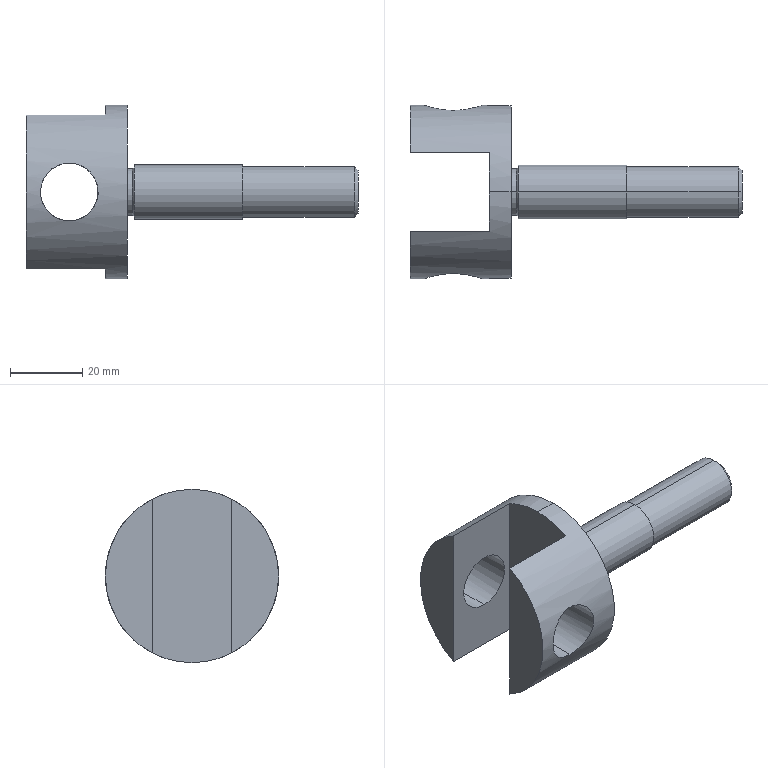Part | SolidWorks | features ICE 2, Chamfer 1, RevCut 1, Revolution 1 | 1 solid | 30 faces | box 92 x 48 x 48 mm | volume 33624 mm3 | cylinder 12 | plane 10 | cone 6 | torus 2 | commonest cylinder face diameters 16 x4 13 x2 14 x2 15 x2 48 x2
STEP:
#1=CARTESIAN_POINT('',(92.,0.,-6.));
#2=VERTEX_POINT('',#1);
#3=CARTESIAN_POINT('',(92.,0.,6.));
#4=VERTEX_POINT('',#3);
#5=CARTESIAN_POINT('',(92.,0.,0.));
#6=DIRECTION('',(1.,0.,0.));
#7=DIRECTION('',(0.,0.,1.));
#8=AXIS2_PLACEMENT_3D('',#5,#6,#7);
#9=CIRCLE('',#8,6.);
#10=EDGE_CURVE('',#2,#4,#9,.T.);
#11=ORIENTED_EDGE('',*,*,#10,.F.);
#12=CARTESIAN_POINT('',(91.,0.,-7.));
#13=VERTEX_POINT('',#12);
#14=CARTESIAN_POINT('',(91.,0.,-7.));
#15=DIRECTION('',(-0.7071,0.,-0.7071));
#16=VECTOR('',#15,1000.);
#17=LINE('',#14,#16);
#18=EDGE_CURVE('',#2,#13,#17,.T.);
#19=ORIENTED_EDGE('',*,*,#18,.T.);
#20=CARTESIAN_POINT('',(91.,0.,7.));
#21=VERTEX_POINT('',#20);
#22=CARTESIAN_POINT('',(91.,0.,0.));
#23=DIRECTION('',(-1.,0.,0.));
#24=DIRECTION('',(0.,0.,1.));
#25=AXIS2_PLACEMENT_3D('',#22,#23,#24);
#26=CIRCLE('',#25,7.);
#27=EDGE_CURVE('',#21,#13,#26,.T.);
#28=ORIENTED_EDGE('',*,*,#27,.F.);
#29=CARTESIAN_POINT('',(91.,0.,7.));
#30=DIRECTION('',(-0.7071,0.,0.7071));
#31=VECTOR('',#30,1000.);
#32=LINE('',#29,#31);
#33=EDGE_CURVE('',#4,#21,#32,.T.);
#34=ORIENTED_EDGE('',*,*,#33,.F.);
#35=EDGE_LOOP('',(#11,#19,#28,#34));
#36=FACE_OUTER_BOUND('',#35,.T.);
#37=CARTESIAN_POINT('',(91.,0.,0.));
#38=DIRECTION('',(-1.,0.,0.));
#39=DIRECTION('',(0.,0.,1.));
#40=AXIS2_PLACEMENT_3D('',#37,#38,#39);
#41=CONICAL_SURFACE('',#40,7.,0.7854);
#42=ADVANCED_FACE('',(#36),#41,.T.);
#43=CARTESIAN_POINT('',(12.,22.627,-8.));
#44=VERTEX_POINT('',#43);
#45=CARTESIAN_POINT('',(12.,22.627,8.));
#46=VERTEX_POINT('',#45);
#47=CARTESIAN_POINT('',(12.,22.627,-8.));
#48=CARTESIAN_POINT('',(11.467,22.627,-8.));
#49=CARTESIAN_POINT('',(10.944,22.646,-7.947));
#50=CARTESIAN_POINT('',(10.174,22.7,-7.793));
#51=CARTESIAN_POINT('',(9.919,22.722,-7.729));
#52=CARTESIAN_POINT('',(9.414,22.773,-7.575));
#53=CARTESIAN_POINT('',(9.165,22.803,-7.485));
#54=CARTESIAN_POINT('',(8.44,22.901,-7.183));
#55=CARTESIAN_POINT('',(7.982,22.977,-6.937));
#56=CARTESIAN_POINT('',(7.332,23.103,-6.502));
#57=CARTESIAN_POINT('',(7.12,23.147,-6.345));
#58=CARTESIAN_POINT('',(6.717,23.235,-6.013));
#59=CARTESIAN_POINT('',(6.525,23.28,-5.839));
#60=CARTESIAN_POINT('',(5.976,23.413,-5.29));
#61=CARTESIAN_POINT('',(5.646,23.501,-4.889));
#62=CARTESIAN_POINT('',(5.061,23.666,-4.016));
#63=CARTESIAN_POINT('',(4.815,23.74,-3.556));
#64=CARTESIAN_POINT('',(4.515,23.833,-2.835));
#65=CARTESIAN_POINT('',(4.426,23.861,-2.589));
#66=CARTESIAN_POINT('',(4.272,23.91,-2.086));
#67=CARTESIAN_POINT('',(4.207,23.932,-1.828));
#68=CARTESIAN_POINT('',(4.052,23.983,-1.052));
#69=CARTESIAN_POINT('',(4.,24.,-0.5299));
#70=CARTESIAN_POINT('',(4.,24.,0.5225));
#71=CARTESIAN_POINT('',(4.053,23.982,1.057));
#72=CARTESIAN_POINT('',(4.259,23.915,2.086));
#73=CARTESIAN_POINT('',(4.412,23.865,2.587));
#74=CARTESIAN_POINT('',(4.817,23.739,3.561));
#75=CARTESIAN_POINT('',(5.065,23.665,4.023));
#76=CARTESIAN_POINT('',(5.499,23.542,4.67));
#77=CARTESIAN_POINT('',(5.654,23.5,4.878));
#78=CARTESIAN_POINT('',(5.986,23.413,5.282));
#79=CARTESIAN_POINT('',(6.163,23.368,5.477));
#80=CARTESIAN_POINT('',(6.715,23.234,6.029));
#81=CARTESIAN_POINT('',(7.115,23.145,6.357));
#82=CARTESIAN_POINT('',(7.979,22.978,6.936));
#83=CARTESIAN_POINT('',(8.447,22.9,7.187));
#84=CARTESIAN_POINT('',(9.41,22.77,7.587));
#85=CARTESIAN_POINT('',(9.909,22.718,7.74));
#86=CARTESIAN_POINT('',(10.686,22.664,7.896));
#87=CARTESIAN_POINT('',(10.95,22.65,7.935));
#88=CARTESIAN_POINT('',(11.475,22.632,7.987));
#89=CARTESIAN_POINT('',(11.738,22.627,8.));
#90=CARTESIAN_POINT('',(12.,22.627,8.));
#91=B_SPLINE_CURVE_WITH_KNOTS('',3,(#47,#48,#49,#50,#51,#52,#53,#54,#55,#56,#57,#58,#59,#60,#61,#62,#63,#64,#65,#66,#67,#68,#69,#70,#71,#72,#73,#74,#75,#76,#77,#78,#79,#80,#81,#82,#83,#84,#85,#86,#87,#88,#89,#90),.UNSPECIFIED.,.F.,.F.,(4,2,2,2,2,2,2,2,2,2,2,2,2,2,2,2,2,2,2,2,2,4),(0.,0.001575,0.002362,0.003149,0.004724,0.005511,0.006298,0.007873,0.009447,0.01023,0.01102,0.0126,0.01417,0.01575,0.01732,0.01811,0.01889,0.02047,0.02204,0.02362,0.02441,0.02519),.UNSPECIFIED.);
#92=EDGE_CURVE('',#44,#46,#91,.T.);
#93=ORIENTED_EDGE('',*,*,#92,.F.);
#94=CARTESIAN_POINT('',(12.,22.627,8.));
#95=CARTESIAN_POINT('',(12.262,22.627,8.));
#96=CARTESIAN_POINT('',(12.524,22.632,7.987));
#97=CARTESIAN_POINT('',(13.049,22.65,7.935));
#98=CARTESIAN_POINT('',(13.312,22.664,7.896));
#99=CARTESIAN_POINT('',(14.09,22.718,7.74));
#100=CARTESIAN_POINT('',(14.591,22.77,7.587));
#101=CARTESIAN_POINT('',(15.556,22.9,7.186));
#102=CARTESIAN_POINT('',(16.023,22.978,6.934));
#103=CARTESIAN_POINT('',(16.886,23.145,6.356));
#104=CARTESIAN_POINT('',(17.287,23.234,6.027));
#105=CARTESIAN_POINT('',(17.841,23.369,5.473));
#106=CARTESIAN_POINT('',(18.018,23.413,5.278));
#107=CARTESIAN_POINT('',(18.348,23.5,4.876));
#108=CARTESIAN_POINT('',(18.502,23.543,4.668));
#109=CARTESIAN_POINT('',(18.791,23.624,4.237));
#110=CARTESIAN_POINT('',(18.925,23.663,4.015));
#111=CARTESIAN_POINT('',(19.172,23.736,3.555));
#112=CARTESIAN_POINT('',(19.285,23.771,3.316));
#113=CARTESIAN_POINT('',(19.589,23.865,2.587));
#114=CARTESIAN_POINT('',(19.741,23.915,2.087));
#115=CARTESIAN_POINT('',(19.895,23.965,1.316));
#116=CARTESIAN_POINT('',(19.934,23.978,1.056));
#117=CARTESIAN_POINT('',(19.987,23.996,0.5287));
#118=CARTESIAN_POINT('',(20.,24.,0.2624));
#119=CARTESIAN_POINT('',(20.,24.,-0.5283));
#120=CARTESIAN_POINT('',(19.948,23.983,-1.05));
#121=CARTESIAN_POINT('',(19.793,23.932,-1.826));
#122=CARTESIAN_POINT('',(19.728,23.911,-2.084));
#123=CARTESIAN_POINT('',(19.574,23.861,-2.588));
#124=CARTESIAN_POINT('',(19.486,23.833,-2.835));
#125=CARTESIAN_POINT('',(19.285,23.771,-3.316));
#126=CARTESIAN_POINT('',(19.173,23.737,-3.552));
#127=CARTESIAN_POINT('',(18.926,23.663,-4.012));
#128=CARTESIAN_POINT('',(18.791,23.624,-4.238));
#129=CARTESIAN_POINT('',(18.353,23.501,-4.891));
#130=CARTESIAN_POINT('',(18.023,23.413,-5.291));
#131=CARTESIAN_POINT('',(17.29,23.235,-6.024));
#132=CARTESIAN_POINT('',(16.881,23.144,-6.36));
#133=CARTESIAN_POINT('',(16.017,22.977,-6.938));
#134=CARTESIAN_POINT('',(15.56,22.901,-7.184));
#135=CARTESIAN_POINT('',(14.835,22.803,-7.486));
#136=CARTESIAN_POINT('',(14.585,22.773,-7.575));
#137=CARTESIAN_POINT('',(14.081,22.721,-7.729));
#138=CARTESIAN_POINT('',(13.826,22.7,-7.793));
#139=CARTESIAN_POINT('',(13.056,22.646,-7.947));
#140=CARTESIAN_POINT('',(12.533,22.627,-8.));
#141=CARTESIAN_POINT('',(12.,22.627,-8.));
#142=B_SPLINE_CURVE_WITH_KNOTS('',3,(#94,#95,#96,#97,#98,#99,#100,#101,#102,#103,#104,#105,#106,#107,#108,#109,#110,#111,#112,#113,#114,#115,#116,#117,#118,#119,#120,#121,#122,#123,#124,#125,#126,#127,#128,#129,#130,#131,#132,#133,#134,#135,#136,#137,#138,#139,#140,#141),.UNSPECIFIED.,.F.,.F.,(4,2,2,2,2,2,2,2,2,2,2,2,2,2,2,2,2,2,2,2,2,2,2,4),(0.02519,0.02598,0.02677,0.02834,0.02991,0.03149,0.03228,0.03306,0.03385,0.03464,0.03621,0.037,0.03779,0.03936,0.04015,0.04093,0.04172,0.04251,0.04408,0.04566,0.04723,0.04802,0.0488,0.05038),.UNSPECIFIED.);
#143=EDGE_CURVE('',#46,#44,#142,.T.);
#144=ORIENTED_EDGE('',*,*,#143,.F.);
#145=EDGE_LOOP('',(#93,#144));
#146=FACE_BOUND('',#145,.T.);
#147=CARTESIAN_POINT('',(28.,0.,24.));
#148=VERTEX_POINT('',#147);
#149=CARTESIAN_POINT('',(28.,0.,-24.));
#150=VERTEX_POINT('',#149);
#151=CARTESIAN_POINT('',(28.,0.,0.));
#152=DIRECTION('',(-1.,0.,0.));
#153=DIRECTION('',(0.,0.,1.));
#154=AXIS2_PLACEMENT_3D('',#151,#152,#153);
#155=CIRCLE('',#154,24.);
#156=EDGE_CURVE('',#148,#150,#155,.T.);
#157=ORIENTED_EDGE('',*,*,#156,.T.);
#158=CARTESIAN_POINT('',(22.,0.,-24.));
#159=VERTEX_POINT('',#158);
#160=CARTESIAN_POINT('',(-36.182,0.,-24.));
#161=DIRECTION('',(-1.,0.,0.));
#162=VECTOR('',#161,1000.);
#163=LINE('',#160,#162);
#164=EDGE_CURVE('',#150,#159,#163,.T.);
#165=ORIENTED_EDGE('',*,*,#164,.T.);
#166=CARTESIAN_POINT('',(22.,11.,-21.331));
#167=VERTEX_POINT('',#166);
#168=CARTESIAN_POINT('',(22.,0.,0.));
#169=DIRECTION('',(-1.,0.,0.));
#170=DIRECTION('',(0.,0.,1.));
#171=AXIS2_PLACEMENT_3D('',#168,#169,#170);
#172=CIRCLE('',#171,24.);
#173=EDGE_CURVE('',#167,#159,#172,.T.);
#174=ORIENTED_EDGE('',*,*,#173,.F.);
#175=CARTESIAN_POINT('',(0.,11.,-21.331));
#176=VERTEX_POINT('',#175);
#177=CARTESIAN_POINT('',(-36.182,11.,-21.331));
#178=DIRECTION('',(-1.,0.,0.));
#179=VECTOR('',#178,1000.);
#180=LINE('',#177,#179);
#181=EDGE_CURVE('',#167,#176,#180,.T.);
#182=ORIENTED_EDGE('',*,*,#181,.T.);
#183=CARTESIAN_POINT('',(0.,11.,21.331));
#184=VERTEX_POINT('',#183);
#185=CARTESIAN_POINT('',(0.,0.,0.));
#186=DIRECTION('',(-1.,0.,0.));
#187=DIRECTION('',(0.,0.,1.));
#188=AXIS2_PLACEMENT_3D('',#185,#186,#187);
#189=CIRCLE('',#188,24.);
#190=EDGE_CURVE('',#184,#176,#189,.T.);
#191=ORIENTED_EDGE('',*,*,#190,.F.);
#192=CARTESIAN_POINT('',(22.,11.,21.331));
#193=VERTEX_POINT('',#192);
#194=CARTESIAN_POINT('',(-36.182,11.,21.331));
#195=DIRECTION('',(1.,0.,0.));
#196=VECTOR('',#195,1000.);
#197=LINE('',#194,#196);
#198=EDGE_CURVE('',#184,#193,#197,.T.);
#199=ORIENTED_EDGE('',*,*,#198,.T.);
#200=CARTESIAN_POINT('',(22.,0.,24.));
#201=VERTEX_POINT('',#200);
#202=CARTESIAN_POINT('',(22.,0.,0.));
#203=DIRECTION('',(-1.,0.,0.));
#204=DIRECTION('',(0.,0.,1.));
#205=AXIS2_PLACEMENT_3D('',#202,#203,#204);
#206=CIRCLE('',#205,24.);
#207=EDGE_CURVE('',#201,#193,#206,.T.);
#208=ORIENTED_EDGE('',*,*,#207,.F.);
#209=CARTESIAN_POINT('',(-36.182,0.,24.));
#210=DIRECTION('',(-1.,0.,0.));
#211=VECTOR('',#210,1000.);
#212=LINE('',#209,#211);
#213=EDGE_CURVE('',#148,#201,#212,.T.);
#214=ORIENTED_EDGE('',*,*,#213,.F.);
#215=EDGE_LOOP('',(#157,#165,#174,#182,#191,#199,#208,#214));
#216=FACE_OUTER_BOUND('',#215,.T.);
#217=CARTESIAN_POINT('',(-36.182,0.,0.));
#218=DIRECTION('',(-1.,0.,0.));
#219=DIRECTION('',(0.,0.,1.));
#220=AXIS2_PLACEMENT_3D('',#217,#218,#219);
#221=CYLINDRICAL_SURFACE('',#220,24.);
#222=ADVANCED_FACE('',(#146,#216),#221,.T.);
#223=CARTESIAN_POINT('',(12.,-11.,-8.));
#224=VERTEX_POINT('',#223);
#225=CARTESIAN_POINT('',(12.,-11.,8.));
#226=VERTEX_POINT('',#225);
#227=CARTESIAN_POINT('',(12.,-11.,0.));
#228=DIRECTION('',(0.,1.,0.));
#229=DIRECTION('',(0.,0.,-1.));
#230=AXIS2_PLACEMENT_3D('',#227,#228,#229);
#231=CIRCLE('',#230,8.);
#232=EDGE_CURVE('',#224,#226,#231,.T.);
#233=ORIENTED_EDGE('',*,*,#232,.T.);
#234=CARTESIAN_POINT('',(12.,-22.627,8.));
#235=VERTEX_POINT('',#234);
#236=CARTESIAN_POINT('',(12.,40.,8.));
#237=DIRECTION('',(0.,-1.,0.));
#238=VECTOR('',#237,1000.);
#239=LINE('',#236,#238);
#240=EDGE_CURVE('',#226,#235,#239,.T.);
#241=ORIENTED_EDGE('',*,*,#240,.T.);
#242=CARTESIAN_POINT('',(12.,-22.627,-8.));
#243=VERTEX_POINT('',#242);
#244=CARTESIAN_POINT('',(12.,-22.627,8.));
#245=CARTESIAN_POINT('',(11.738,-22.627,8.));
#246=CARTESIAN_POINT('',(11.476,-22.632,7.987));
#247=CARTESIAN_POINT('',(10.951,-22.65,7.935));
#248=CARTESIAN_POINT('',(10.688,-22.664,7.896));
#249=CARTESIAN_POINT('',(9.91,-22.718,7.74));
#250=CARTESIAN_POINT('',(9.409,-22.77,7.587));
#251=CARTESIAN_POINT('',(8.444,-22.9,7.186));
#252=CARTESIAN_POINT('',(7.977,-22.978,6.934));
#253=CARTESIAN_POINT('',(7.114,-23.145,6.356));
#254=CARTESIAN_POINT('',(6.713,-23.234,6.027));
#255=CARTESIAN_POINT('',(6.159,-23.369,5.473));
#256=CARTESIAN_POINT('',(5.982,-23.413,5.278));
#257=CARTESIAN_POINT('',(5.652,-23.5,4.876));
#258=CARTESIAN_POINT('',(5.498,-23.543,4.668));
#259=CARTESIAN_POINT('',(5.209,-23.624,4.237));
#260=CARTESIAN_POINT('',(5.075,-23.663,4.015));
#261=CARTESIAN_POINT('',(4.828,-23.736,3.555));
#262=CARTESIAN_POINT('',(4.715,-23.771,3.316));
#263=CARTESIAN_POINT('',(4.411,-23.865,2.587));
#264=CARTESIAN_POINT('',(4.259,-23.915,2.087));
#265=CARTESIAN_POINT('',(4.105,-23.965,1.316));
#266=CARTESIAN_POINT('',(4.066,-23.978,1.056));
#267=CARTESIAN_POINT('',(4.013,-23.996,0.5287));
#268=CARTESIAN_POINT('',(4.,-24.,0.2624));
#269=CARTESIAN_POINT('',(4.,-24.,-0.5283));
#270=CARTESIAN_POINT('',(4.052,-23.983,-1.05));
#271=CARTESIAN_POINT('',(4.207,-23.932,-1.826));
#272=CARTESIAN_POINT('',(4.272,-23.911,-2.084));
#273=CARTESIAN_POINT('',(4.426,-23.861,-2.588));
#274=CARTESIAN_POINT('',(4.514,-23.833,-2.835));
#275=CARTESIAN_POINT('',(4.715,-23.771,-3.316));
#276=CARTESIAN_POINT('',(4.827,-23.737,-3.552));
#277=CARTESIAN_POINT('',(5.074,-23.663,-4.012));
#278=CARTESIAN_POINT('',(5.209,-23.624,-4.238));
#279=CARTESIAN_POINT('',(5.647,-23.501,-4.891));
#280=CARTESIAN_POINT('',(5.977,-23.413,-5.291));
#281=CARTESIAN_POINT('',(6.71,-23.235,-6.024));
#282=CARTESIAN_POINT('',(7.119,-23.144,-6.36));
#283=CARTESIAN_POINT('',(7.983,-22.977,-6.938));
#284=CARTESIAN_POINT('',(8.44,-22.901,-7.184));
#285=CARTESIAN_POINT('',(9.165,-22.803,-7.486));
#286=CARTESIAN_POINT('',(9.415,-22.773,-7.575));
#287=CARTESIAN_POINT('',(9.919,-22.721,-7.729));
#288=CARTESIAN_POINT('',(10.174,-22.7,-7.793));
#289=CARTESIAN_POINT('',(10.944,-22.646,-7.947));
#290=CARTESIAN_POINT('',(11.467,-22.627,-8.));
#291=CARTESIAN_POINT('',(12.,-22.627,-8.));
#292=B_SPLINE_CURVE_WITH_KNOTS('',3,(#244,#245,#246,#247,#248,#249,#250,#251,#252,#253,#254,#255,#256,#257,#258,#259,#260,#261,#262,#263,#264,#265,#266,#267,#268,#269,#270,#271,#272,#273,#274,#275,#276,#277,#278,#279,#280,#281,#282,#283,#284,#285,#286,#287,#288,#289,#290,#291),.UNSPECIFIED.,.F.,.F.,(4,2,2,2,2,2,2,2,2,2,2,2,2,2,2,2,2,2,2,2,2,2,2,4),(0.02519,0.02598,0.02677,0.02834,0.02991,0.03149,0.03228,0.03306,0.03385,0.03464,0.03621,0.037,0.03779,0.03936,0.04015,0.04093,0.04172,0.04251,0.04408,0.04566,0.04723,0.04802,0.0488,0.05038),.UNSPECIFIED.);
#293=EDGE_CURVE('',#235,#243,#292,.T.);
#294=ORIENTED_EDGE('',*,*,#293,.T.);
#295=CARTESIAN_POINT('',(12.,40.,-8.));
#296=DIRECTION('',(0.,-1.,0.));
#297=VECTOR('',#296,1000.);
#298=LINE('',#295,#297);
#299=EDGE_CURVE('',#224,#243,#298,.T.);
#300=ORIENTED_EDGE('',*,*,#299,.F.);
#301=EDGE_LOOP('',(#233,#241,#294,#300));
#302=FACE_OUTER_BOUND('',#301,.T.);
#303=CARTESIAN_POINT('',(12.,40.,0.));
#304=DIRECTION('',(0.,-1.,0.));
#305=DIRECTION('',(0.,0.,-1.));
#306=AXIS2_PLACEMENT_3D('',#303,#304,#305);
#307=CYLINDRICAL_SURFACE('',#306,8.);
#308=ADVANCED_FACE('',(#302),#307,.F.);
#309=ORIENTED_EDGE('',*,*,#92,.T.);
#310=CARTESIAN_POINT('',(12.,11.,8.));
#311=VERTEX_POINT('',#310);
#312=CARTESIAN_POINT('',(12.,40.,8.));
#313=DIRECTION('',(0.,-1.,0.));
#314=VECTOR('',#313,1000.);
#315=LINE('',#312,#314);
#316=EDGE_CURVE('',#46,#311,#315,.T.);
#317=ORIENTED_EDGE('',*,*,#316,.T.);
#318=CARTESIAN_POINT('',(12.,11.,-8.));
#319=VERTEX_POINT('',#318);
#320=CARTESIAN_POINT('',(12.,11.,0.));
#321=DIRECTION('',(0.,-1.,0.));
#322=DIRECTION('',(0.,0.,1.));
#323=AXIS2_PLACEMENT_3D('',#320,#321,#322);
#324=CIRCLE('',#323,8.);
#325=EDGE_CURVE('',#311,#319,#324,.T.);
#326=ORIENTED_EDGE('',*,*,#325,.T.);
#327=CARTESIAN_POINT('',(12.,40.,-8.));
#328=DIRECTION('',(0.,-1.,0.));
#329=VECTOR('',#328,1000.);
#330=LINE('',#327,#329);
#331=EDGE_CURVE('',#44,#319,#330,.T.);
#332=ORIENTED_EDGE('',*,*,#331,.F.);
#333=EDGE_LOOP('',(#309,#317,#326,#332));
#334=FACE_OUTER_BOUND('',#333,.T.);
#335=CARTESIAN_POINT('',(12.,40.,0.));
#336=DIRECTION('',(0.,-1.,0.));
#337=DIRECTION('',(0.,0.,-1.));
#338=AXIS2_PLACEMENT_3D('',#335,#336,#337);
#339=CYLINDRICAL_SURFACE('',#338,8.);
#340=ADVANCED_FACE('',(#334),#339,.F.);
#341=CARTESIAN_POINT('',(27.5,0.,-7.));
#342=VERTEX_POINT('',#341);
#343=CARTESIAN_POINT('',(27.5,0.,7.));
#344=VERTEX_POINT('',#343);
#345=CARTESIAN_POINT('',(27.5,0.,0.));
#346=DIRECTION('',(-1.,0.,0.));
#347=DIRECTION('',(0.,0.,1.));
#348=AXIS2_PLACEMENT_3D('',#345,#346,#347);
#349=CIRCLE('',#348,7.);
#350=EDGE_CURVE('',#342,#344,#349,.T.);
#351=ORIENTED_EDGE('',*,*,#350,.F.);
#352=CARTESIAN_POINT('',(28.,0.,-6.5));
#353=VERTEX_POINT('',#352);
#354=CARTESIAN_POINT('',(28.,0.,-7.));
#355=DIRECTION('',(0.,1.,0.));
#356=DIRECTION('',(0.,0.,1.));
#357=AXIS2_PLACEMENT_3D('',#354,#355,#356);
#358=CIRCLE('',#357,0.5);
#359=EDGE_CURVE('',#342,#353,#358,.T.);
#360=ORIENTED_EDGE('',*,*,#359,.T.);
#361=CARTESIAN_POINT('',(28.,0.,6.5));
#362=VERTEX_POINT('',#361);
#363=CARTESIAN_POINT('',(28.,0.,0.));
#364=DIRECTION('',(-1.,0.,0.));
#365=DIRECTION('',(0.,0.,1.));
#366=AXIS2_PLACEMENT_3D('',#363,#364,#365);
#367=CIRCLE('',#366,6.5);
#368=EDGE_CURVE('',#353,#362,#367,.T.);
#369=ORIENTED_EDGE('',*,*,#368,.T.);
#370=CARTESIAN_POINT('',(28.,0.,7.));
#371=DIRECTION('',(0.,-1.,0.));
#372=DIRECTION('',(0.,0.,-1.));
#373=AXIS2_PLACEMENT_3D('',#370,#371,#372);
#374=CIRCLE('',#373,0.5);
#375=EDGE_CURVE('',#344,#362,#374,.T.);
#376=ORIENTED_EDGE('',*,*,#375,.F.);
#377=EDGE_LOOP('',(#351,#360,#369,#376));
#378=FACE_OUTER_BOUND('',#377,.T.);
#379=CARTESIAN_POINT('',(28.,0.,0.));
#380=DIRECTION('',(-1.,0.,0.));
#381=DIRECTION('',(0.,0.,1.));
#382=AXIS2_PLACEMENT_3D('',#379,#380,#381);
#383=TOROIDAL_SURFACE('',#382,7.,0.5);
#384=ADVANCED_FACE('',(#378),#383,.F.);
#385=CARTESIAN_POINT('',(27.5,0.,-8.));
#386=VERTEX_POINT('',#385);
#387=CARTESIAN_POINT('',(27.5,0.,8.));
#388=VERTEX_POINT('',#387);
#389=CARTESIAN_POINT('',(27.5,0.,0.));
#390=DIRECTION('',(-1.,0.,0.));
#391=DIRECTION('',(0.,0.,1.));
#392=AXIS2_PLACEMENT_3D('',#389,#390,#391);
#393=CIRCLE('',#392,8.);
#394=EDGE_CURVE('',#386,#388,#393,.T.);
#395=ORIENTED_EDGE('',*,*,#394,.T.);
#396=CARTESIAN_POINT('',(28.,0.,8.5));
#397=VERTEX_POINT('',#396);
#398=CARTESIAN_POINT('',(27.5,0.,8.));
#399=DIRECTION('',(0.7071,0.,0.7071));
#400=VECTOR('',#399,1000.);
#401=LINE('',#398,#400);
#402=EDGE_CURVE('',#388,#397,#401,.T.);
#403=ORIENTED_EDGE('',*,*,#402,.T.);
#404=CARTESIAN_POINT('',(28.,0.,-8.5));
#405=VERTEX_POINT('',#404);
#406=CARTESIAN_POINT('',(28.,0.,0.));
#407=DIRECTION('',(-1.,0.,0.));
#408=DIRECTION('',(0.,0.,1.));
#409=AXIS2_PLACEMENT_3D('',#406,#407,#408);
#410=CIRCLE('',#409,8.5);
#411=EDGE_CURVE('',#405,#397,#410,.T.);
#412=ORIENTED_EDGE('',*,*,#411,.F.);
#413=CARTESIAN_POINT('',(27.5,0.,-8.));
#414=DIRECTION('',(0.7071,0.,-0.7071));
#415=VECTOR('',#414,1000.);
#416=LINE('',#413,#415);
#417=EDGE_CURVE('',#386,#405,#416,.T.);
#418=ORIENTED_EDGE('',*,*,#417,.F.);
#419=EDGE_LOOP('',(#395,#403,#412,#418));
#420=FACE_OUTER_BOUND('',#419,.T.);
#421=CARTESIAN_POINT('',(27.5,0.,0.));
#422=DIRECTION('',(1.,0.,0.));
#423=DIRECTION('',(0.,0.,-1.));
#424=AXIS2_PLACEMENT_3D('',#421,#422,#423);
#425=CONICAL_SURFACE('',#424,8.,0.7854);
#426=ADVANCED_FACE('',(#420),#425,.F.);
#427=CARTESIAN_POINT('',(29.5,0.,6.5));
#428=VERTEX_POINT('',#427);
#429=CARTESIAN_POINT('',(29.5,0.,-6.5));
#430=VERTEX_POINT('',#429);
#431=CARTESIAN_POINT('',(29.5,0.,0.));
#432=DIRECTION('',(-1.,0.,0.));
#433=DIRECTION('',(0.,0.,1.));
#434=AXIS2_PLACEMENT_3D('',#431,#432,#433);
#435=CIRCLE('',#434,6.5);
#436=EDGE_CURVE('',#428,#430,#435,.T.);
#437=ORIENTED_EDGE('',*,*,#436,.F.);
#438=CARTESIAN_POINT('',(30.,0.,7.));
#439=VERTEX_POINT('',#438);
#440=CARTESIAN_POINT('',(29.5,0.,6.5));
#441=DIRECTION('',(0.7071,0.,0.7071));
#442=VECTOR('',#441,1000.);
#443=LINE('',#440,#442);
#444=EDGE_CURVE('',#428,#439,#443,.T.);
#445=ORIENTED_EDGE('',*,*,#444,.T.);
#446=CARTESIAN_POINT('',(30.,0.,-7.));
#447=VERTEX_POINT('',#446);
#448=CARTESIAN_POINT('',(30.,0.,0.));
#449=DIRECTION('',(-1.,0.,0.));
#450=DIRECTION('',(0.,0.,1.));
#451=AXIS2_PLACEMENT_3D('',#448,#449,#450);
#452=CIRCLE('',#451,7.);
#453=EDGE_CURVE('',#439,#447,#452,.T.);
#454=ORIENTED_EDGE('',*,*,#453,.T.);
#455=CARTESIAN_POINT('',(29.5,0.,-6.5));
#456=DIRECTION('',(0.7071,0.,-0.7071));
#457=VECTOR('',#456,1000.);
#458=LINE('',#455,#457);
#459=EDGE_CURVE('',#430,#447,#458,.T.);
#460=ORIENTED_EDGE('',*,*,#459,.F.);
#461=EDGE_LOOP('',(#437,#445,#454,#460));
#462=FACE_OUTER_BOUND('',#461,.T.);
#463=CARTESIAN_POINT('',(29.5,0.,0.));
#464=DIRECTION('',(1.,0.,0.));
#465=DIRECTION('',(0.,0.,-1.));
#466=AXIS2_PLACEMENT_3D('',#463,#464,#465);
#467=CONICAL_SURFACE('',#466,6.5,0.7854);
#468=ADVANCED_FACE('',(#462),#467,.T.);
#469=ORIENTED_EDGE('',*,*,#436,.T.);
#470=CARTESIAN_POINT('',(0.,0.,-6.5));
#471=DIRECTION('',(-1.,0.,0.));
#472=VECTOR('',#471,1000.);
#473=LINE('',#470,#472);
#474=EDGE_CURVE('',#430,#353,#473,.T.);
#475=ORIENTED_EDGE('',*,*,#474,.T.);
#476=CARTESIAN_POINT('',(28.,0.,0.));
#477=DIRECTION('',(-1.,0.,0.));
#478=DIRECTION('',(0.,0.,1.));
#479=AXIS2_PLACEMENT_3D('',#476,#477,#478);
#480=CIRCLE('',#479,6.5);
#481=EDGE_CURVE('',#362,#353,#480,.T.);
#482=ORIENTED_EDGE('',*,*,#481,.F.);
#483=CARTESIAN_POINT('',(0.,0.,6.5));
#484=DIRECTION('',(-1.,0.,0.));
#485=VECTOR('',#484,1000.);
#486=LINE('',#483,#485);
#487=EDGE_CURVE('',#428,#362,#486,.T.);
#488=ORIENTED_EDGE('',*,*,#487,.F.);
#489=EDGE_LOOP('',(#469,#475,#482,#488));
#490=FACE_OUTER_BOUND('',#489,.T.);
#491=CARTESIAN_POINT('',(0.,0.,0.));
#492=DIRECTION('',(-1.,0.,0.));
#493=DIRECTION('',(0.,0.,1.));
#494=AXIS2_PLACEMENT_3D('',#491,#492,#493);
#495=CYLINDRICAL_SURFACE('',#494,6.5);
#496=ADVANCED_FACE('',(#490),#495,.T.);
#497=ORIENTED_EDGE('',*,*,#27,.T.);
#498=CARTESIAN_POINT('',(60.,0.,-7.));
#499=VERTEX_POINT('',#498);
#500=CARTESIAN_POINT('',(-36.182,0.,-7.));
#501=DIRECTION('',(-1.,0.,0.));
#502=VECTOR('',#501,1000.);
#503=LINE('',#500,#502);
#504=EDGE_CURVE('',#13,#499,#503,.T.);
#505=ORIENTED_EDGE('',*,*,#504,.T.);
#506=CARTESIAN_POINT('',(60.,0.,7.));
#507=VERTEX_POINT('',#506);
#508=CARTESIAN_POINT('',(60.,0.,0.));
#509=DIRECTION('',(-1.,0.,0.));
#510=DIRECTION('',(0.,0.,1.));
#511=AXIS2_PLACEMENT_3D('',#508,#509,#510);
#512=CIRCLE('',#511,7.);
#513=EDGE_CURVE('',#507,#499,#512,.T.);
#514=ORIENTED_EDGE('',*,*,#513,.F.);
#515=CARTESIAN_POINT('',(-36.182,0.,7.));
#516=DIRECTION('',(-1.,0.,0.));
#517=VECTOR('',#516,1000.);
#518=LINE('',#515,#517);
#519=EDGE_CURVE('',#21,#507,#518,.T.);
#520=ORIENTED_EDGE('',*,*,#519,.F.);
#521=EDGE_LOOP('',(#497,#505,#514,#520));
#522=FACE_OUTER_BOUND('',#521,.T.);
#523=CARTESIAN_POINT('',(-36.182,0.,0.));
#524=DIRECTION('',(-1.,0.,0.));
#525=DIRECTION('',(0.,0.,1.));
#526=AXIS2_PLACEMENT_3D('',#523,#524,#525);
#527=CYLINDRICAL_SURFACE('',#526,7.);
#528=ADVANCED_FACE('',(#522),#527,.T.);
#529=CARTESIAN_POINT('',(60.,0.,7.5));
#530=VERTEX_POINT('',#529);
#531=CARTESIAN_POINT('',(60.,0.,-7.5));
#532=VERTEX_POINT('',#531);
#533=CARTESIAN_POINT('',(60.,0.,0.));
#534=DIRECTION('',(-1.,0.,0.));
#535=DIRECTION('',(0.,0.,1.));
#536=AXIS2_PLACEMENT_3D('',#533,#534,#535);
#537=CIRCLE('',#536,7.5);
#538=EDGE_CURVE('',#530,#532,#537,.T.);
#539=ORIENTED_EDGE('',*,*,#538,.T.);
#540=CARTESIAN_POINT('',(30.,0.,-7.5));
#541=VERTEX_POINT('',#540);
#542=CARTESIAN_POINT('',(-36.182,0.,-7.5));
#543=DIRECTION('',(-1.,0.,0.));
#544=VECTOR('',#543,1000.);
#545=LINE('',#542,#544);
#546=EDGE_CURVE('',#532,#541,#545,.T.);
#547=ORIENTED_EDGE('',*,*,#546,.T.);
#548=CARTESIAN_POINT('',(30.,0.,7.5));
#549=VERTEX_POINT('',#548);
#550=CARTESIAN_POINT('',(30.,0.,0.));
#551=DIRECTION('',(-1.,0.,0.));
#552=DIRECTION('',(0.,0.,1.));
#553=AXIS2_PLACEMENT_3D('',#550,#551,#552);
#554=CIRCLE('',#553,7.5);
#555=EDGE_CURVE('',#549,#541,#554,.T.);
#556=ORIENTED_EDGE('',*,*,#555,.F.);
#557=CARTESIAN_POINT('',(-36.182,0.,7.5));
#558=DIRECTION('',(-1.,0.,0.));
#559=VECTOR('',#558,1000.);
#560=LINE('',#557,#559);
#561=EDGE_CURVE('',#530,#549,#560,.T.);
#562=ORIENTED_EDGE('',*,*,#561,.F.);
#563=EDGE_LOOP('',(#539,#547,#556,#562));
#564=FACE_OUTER_BOUND('',#563,.T.);
#565=CARTESIAN_POINT('',(-36.182,0.,0.));
#566=DIRECTION('',(-1.,0.,0.));
#567=DIRECTION('',(0.,0.,1.));
#568=AXIS2_PLACEMENT_3D('',#565,#566,#567);
#569=CYLINDRICAL_SURFACE('',#568,7.5);
#570=ADVANCED_FACE('',(#564),#569,.T.);
#571=CARTESIAN_POINT('',(30.,0.,0.));
#572=DIRECTION('',(-1.,0.,0.));
#573=DIRECTION('',(0.,0.,1.));
#574=AXIS2_PLACEMENT_3D('',#571,#572,#573);
#575=CIRCLE('',#574,7.);
#576=EDGE_CURVE('',#447,#439,#575,.T.);
#577=ORIENTED_EDGE('',*,*,#576,.F.);
#578=ORIENTED_EDGE('',*,*,#453,.F.);
#579=EDGE_LOOP('',(#577,#578));
#580=FACE_BOUND('',#579,.T.);
#581=ORIENTED_EDGE('',*,*,#555,.T.);
#582=CARTESIAN_POINT('',(30.,0.,0.));
#583=DIRECTION('',(-1.,0.,0.));
#584=DIRECTION('',(0.,0.,1.));
#585=AXIS2_PLACEMENT_3D('',#582,#583,#584);
#586=CIRCLE('',#585,7.5);
#587=EDGE_CURVE('',#541,#549,#586,.T.);
#588=ORIENTED_EDGE('',*,*,#587,.T.);
#589=EDGE_LOOP('',(#581,#588));
#590=FACE_OUTER_BOUND('',#589,.T.);
#591=CARTESIAN_POINT('',(30.,7.,0.));
#592=DIRECTION('',(1.,0.,0.));
#593=DIRECTION('',(0.,0.,-1.));
#594=AXIS2_PLACEMENT_3D('',#591,#592,#593);
#595=PLANE('',#594);
#596=ADVANCED_FACE('',(#580,#590),#595,.F.);
#597=ORIENTED_EDGE('',*,*,#546,.F.);
#598=CARTESIAN_POINT('',(60.,0.,0.));
#599=DIRECTION('',(-1.,0.,0.));
#600=DIRECTION('',(0.,0.,1.));
#601=AXIS2_PLACEMENT_3D('',#598,#599,#600);
#602=CIRCLE('',#601,7.5);
#603=EDGE_CURVE('',#532,#530,#602,.T.);
#604=ORIENTED_EDGE('',*,*,#603,.T.);
#605=ORIENTED_EDGE('',*,*,#561,.T.);
#606=ORIENTED_EDGE('',*,*,#587,.F.);
#607=EDGE_LOOP('',(#597,#604,#605,#606));
#608=FACE_OUTER_BOUND('',#607,.T.);
#609=CARTESIAN_POINT('',(-36.182,0.,0.));
#610=DIRECTION('',(-1.,0.,0.));
#611=DIRECTION('',(0.,0.,1.));
#612=AXIS2_PLACEMENT_3D('',#609,#610,#611);
#613=CYLINDRICAL_SURFACE('',#612,7.5);
#614=ADVANCED_FACE('',(#608),#613,.T.);
#615=ORIENTED_EDGE('',*,*,#538,.F.);
#616=ORIENTED_EDGE('',*,*,#603,.F.);
#617=EDGE_LOOP('',(#615,#616));
#618=FACE_OUTER_BOUND('',#617,.T.);
#619=ORIENTED_EDGE('',*,*,#513,.T.);
#620=CARTESIAN_POINT('',(60.,0.,0.));
#621=DIRECTION('',(-1.,0.,0.));
#622=DIRECTION('',(0.,0.,1.));
#623=AXIS2_PLACEMENT_3D('',#620,#621,#622);
#624=CIRCLE('',#623,7.);
#625=EDGE_CURVE('',#499,#507,#624,.T.);
#626=ORIENTED_EDGE('',*,*,#625,.T.);
#627=EDGE_LOOP('',(#619,#626));
#628=FACE_BOUND('',#627,.T.);
#629=CARTESIAN_POINT('',(60.,7.5,0.));
#630=DIRECTION('',(-1.,0.,0.));
#631=DIRECTION('',(0.,0.,1.));
#632=AXIS2_PLACEMENT_3D('',#629,#630,#631);
#633=PLANE('',#632);
#634=ADVANCED_FACE('',(#618,#628),#633,.F.);
#635=ORIENTED_EDGE('',*,*,#504,.F.);
#636=CARTESIAN_POINT('',(91.,0.,0.));
#637=DIRECTION('',(-1.,0.,0.));
#638=DIRECTION('',(0.,0.,1.));
#639=AXIS2_PLACEMENT_3D('',#636,#637,#638);
#640=CIRCLE('',#639,7.);
#641=EDGE_CURVE('',#13,#21,#640,.T.);
#642=ORIENTED_EDGE('',*,*,#641,.T.);
#643=ORIENTED_EDGE('',*,*,#519,.T.);
#644=ORIENTED_EDGE('',*,*,#625,.F.);
#645=EDGE_LOOP('',(#635,#642,#643,#644));
#646=FACE_OUTER_BOUND('',#645,.T.);
#647=CARTESIAN_POINT('',(-36.182,0.,0.));
#648=DIRECTION('',(-1.,0.,0.));
#649=DIRECTION('',(0.,0.,1.));
#650=AXIS2_PLACEMENT_3D('',#647,#648,#649);
#651=CYLINDRICAL_SURFACE('',#650,7.);
#652=ADVANCED_FACE('',(#646),#651,.T.);
#653=CARTESIAN_POINT('',(92.,0.,0.));
#654=DIRECTION('',(1.,0.,0.));
#655=DIRECTION('',(0.,0.,1.));
#656=AXIS2_PLACEMENT_3D('',#653,#654,#655);
#657=CIRCLE('',#656,6.);
#658=EDGE_CURVE('',#4,#2,#657,.T.);
#659=ORIENTED_EDGE('',*,*,#658,.T.);
#660=ORIENTED_EDGE('',*,*,#10,.T.);
#661=EDGE_LOOP('',(#659,#660));
#662=FACE_OUTER_BOUND('',#661,.T.);
#663=CARTESIAN_POINT('',(92.,7.,0.));
#664=DIRECTION('',(-1.,0.,0.));
#665=DIRECTION('',(0.,0.,1.));
#666=AXIS2_PLACEMENT_3D('',#663,#664,#665);
#667=PLANE('',#666);
#668=ADVANCED_FACE('',(#662),#667,.F.);
#669=ORIENTED_EDGE('',*,*,#444,.F.);
#670=CARTESIAN_POINT('',(29.5,0.,0.));
#671=DIRECTION('',(-1.,0.,0.));
#672=DIRECTION('',(0.,0.,1.));
#673=AXIS2_PLACEMENT_3D('',#670,#671,#672);
#674=CIRCLE('',#673,6.5);
#675=EDGE_CURVE('',#430,#428,#674,.T.);
#676=ORIENTED_EDGE('',*,*,#675,.F.);
#677=ORIENTED_EDGE('',*,*,#459,.T.);
#678=ORIENTED_EDGE('',*,*,#576,.T.);
#679=EDGE_LOOP('',(#669,#676,#677,#678));
#680=FACE_OUTER_BOUND('',#679,.T.);
#681=CARTESIAN_POINT('',(29.5,0.,0.));
#682=DIRECTION('',(1.,0.,0.));
#683=DIRECTION('',(0.,0.,-1.));
#684=AXIS2_PLACEMENT_3D('',#681,#682,#683);
#685=CONICAL_SURFACE('',#684,6.5,0.7854);
#686=ADVANCED_FACE('',(#680),#685,.T.);
#687=ORIENTED_EDGE('',*,*,#474,.F.);
#688=ORIENTED_EDGE('',*,*,#675,.T.);
#689=ORIENTED_EDGE('',*,*,#487,.T.);
#690=ORIENTED_EDGE('',*,*,#368,.F.);
#691=EDGE_LOOP('',(#687,#688,#689,#690));
#692=FACE_OUTER_BOUND('',#691,.T.);
#693=CARTESIAN_POINT('',(0.,0.,0.));
#694=DIRECTION('',(-1.,0.,0.));
#695=DIRECTION('',(0.,0.,1.));
#696=AXIS2_PLACEMENT_3D('',#693,#694,#695);
#697=CYLINDRICAL_SURFACE('',#696,6.5);
#698=ADVANCED_FACE('',(#692),#697,.T.);
#699=ORIENTED_EDGE('',*,*,#402,.F.);
#700=CARTESIAN_POINT('',(27.5,0.,0.));
#701=DIRECTION('',(-1.,0.,0.));
#702=DIRECTION('',(0.,0.,1.));
#703=AXIS2_PLACEMENT_3D('',#700,#701,#702);
#704=CIRCLE('',#703,8.);
#705=EDGE_CURVE('',#388,#386,#704,.T.);
#706=ORIENTED_EDGE('',*,*,#705,.T.);
#707=ORIENTED_EDGE('',*,*,#417,.T.);
#708=CARTESIAN_POINT('',(28.,0.,0.));
#709=DIRECTION('',(-1.,0.,0.));
#710=DIRECTION('',(0.,0.,1.));
#711=AXIS2_PLACEMENT_3D('',#708,#709,#710);
#712=CIRCLE('',#711,8.5);
#713=EDGE_CURVE('',#397,#405,#712,.T.);
#714=ORIENTED_EDGE('',*,*,#713,.F.);
#715=EDGE_LOOP('',(#699,#706,#707,#714));
#716=FACE_OUTER_BOUND('',#715,.T.);
#717=CARTESIAN_POINT('',(27.5,0.,0.));
#718=DIRECTION('',(1.,0.,0.));
#719=DIRECTION('',(0.,0.,-1.));
#720=AXIS2_PLACEMENT_3D('',#717,#718,#719);
#721=CONICAL_SURFACE('',#720,8.,0.7854);
#722=ADVANCED_FACE('',(#716),#721,.F.);
#723=ORIENTED_EDGE('',*,*,#394,.F.);
#724=ORIENTED_EDGE('',*,*,#705,.F.);
#725=EDGE_LOOP('',(#723,#724));
#726=FACE_OUTER_BOUND('',#725,.T.);
#727=CARTESIAN_POINT('',(27.5,0.,0.));
#728=DIRECTION('',(-1.,0.,0.));
#729=DIRECTION('',(0.,0.,1.));
#730=AXIS2_PLACEMENT_3D('',#727,#728,#729);
#731=CIRCLE('',#730,7.);
#732=EDGE_CURVE('',#344,#342,#731,.T.);
#733=ORIENTED_EDGE('',*,*,#732,.T.);
#734=ORIENTED_EDGE('',*,*,#350,.T.);
#735=EDGE_LOOP('',(#733,#734));
#736=FACE_BOUND('',#735,.T.);
#737=CARTESIAN_POINT('',(27.5,0.,0.));
#738=DIRECTION('',(-1.,0.,0.));
#739=DIRECTION('',(0.,0.,1.));
#740=AXIS2_PLACEMENT_3D('',#737,#738,#739);
#741=PLANE('',#740);
#742=ADVANCED_FACE('',(#726,#736),#741,.F.);
#743=ORIENTED_EDGE('',*,*,#359,.F.);
#744=ORIENTED_EDGE('',*,*,#732,.F.);
#745=ORIENTED_EDGE('',*,*,#375,.T.);
#746=ORIENTED_EDGE('',*,*,#481,.T.);
#747=EDGE_LOOP('',(#743,#744,#745,#746));
#748=FACE_OUTER_BOUND('',#747,.T.);
#749=CARTESIAN_POINT('',(28.,0.,0.));
#750=DIRECTION('',(-1.,0.,0.));
#751=DIRECTION('',(0.,0.,1.));
#752=AXIS2_PLACEMENT_3D('',#749,#750,#751);
#753=TOROIDAL_SURFACE('',#752,7.,0.5);
#754=ADVANCED_FACE('',(#748),#753,.F.);
#755=ORIENTED_EDGE('',*,*,#316,.F.);
#756=ORIENTED_EDGE('',*,*,#143,.T.);
#757=ORIENTED_EDGE('',*,*,#331,.T.);
#758=CARTESIAN_POINT('',(12.,11.,0.));
#759=DIRECTION('',(0.,-1.,0.));
#760=DIRECTION('',(0.,0.,1.));
#761=AXIS2_PLACEMENT_3D('',#758,#759,#760);
#762=CIRCLE('',#761,8.);
#763=EDGE_CURVE('',#319,#311,#762,.T.);
#764=ORIENTED_EDGE('',*,*,#763,.T.);
#765=EDGE_LOOP('',(#755,#756,#757,#764));
#766=FACE_OUTER_BOUND('',#765,.T.);
#767=CARTESIAN_POINT('',(12.,40.,0.));
#768=DIRECTION('',(0.,-1.,0.));
#769=DIRECTION('',(0.,0.,-1.));
#770=AXIS2_PLACEMENT_3D('',#767,#768,#769);
#771=CYLINDRICAL_SURFACE('',#770,8.);
#772=ADVANCED_FACE('',(#766),#771,.F.);
#773=ORIENTED_EDGE('',*,*,#240,.F.);
#774=CARTESIAN_POINT('',(12.,-11.,0.));
#775=DIRECTION('',(0.,1.,0.));
#776=DIRECTION('',(0.,0.,-1.));
#777=AXIS2_PLACEMENT_3D('',#774,#775,#776);
#778=CIRCLE('',#777,8.);
#779=EDGE_CURVE('',#226,#224,#778,.T.);
#780=ORIENTED_EDGE('',*,*,#779,.T.);
#781=ORIENTED_EDGE('',*,*,#299,.T.);
#782=CARTESIAN_POINT('',(12.,-22.627,-8.));
#783=CARTESIAN_POINT('',(12.533,-22.627,-8.));
#784=CARTESIAN_POINT('',(13.056,-22.646,-7.947));
#785=CARTESIAN_POINT('',(13.826,-22.7,-7.793));
#786=CARTESIAN_POINT('',(14.081,-22.722,-7.729));
#787=CARTESIAN_POINT('',(14.586,-22.773,-7.575));
#788=CARTESIAN_POINT('',(14.835,-22.803,-7.485));
#789=CARTESIAN_POINT('',(15.56,-22.901,-7.183));
#790=CARTESIAN_POINT('',(16.018,-22.977,-6.937));
#791=CARTESIAN_POINT('',(16.668,-23.103,-6.502));
#792=CARTESIAN_POINT('',(16.88,-23.147,-6.345));
#793=CARTESIAN_POINT('',(17.283,-23.235,-6.013));
#794=CARTESIAN_POINT('',(17.475,-23.28,-5.839));
#795=CARTESIAN_POINT('',(18.024,-23.413,-5.29));
#796=CARTESIAN_POINT('',(18.354,-23.501,-4.889));
#797=CARTESIAN_POINT('',(18.939,-23.666,-4.016));
#798=CARTESIAN_POINT('',(19.185,-23.74,-3.556));
#799=CARTESIAN_POINT('',(19.485,-23.833,-2.835));
#800=CARTESIAN_POINT('',(19.574,-23.861,-2.589));
#801=CARTESIAN_POINT('',(19.728,-23.91,-2.086));
#802=CARTESIAN_POINT('',(19.793,-23.932,-1.828));
#803=CARTESIAN_POINT('',(19.948,-23.983,-1.052));
#804=CARTESIAN_POINT('',(20.,-24.,-0.5299));
#805=CARTESIAN_POINT('',(20.,-24.,0.5225));
#806=CARTESIAN_POINT('',(19.947,-23.982,1.057));
#807=CARTESIAN_POINT('',(19.741,-23.915,2.086));
#808=CARTESIAN_POINT('',(19.588,-23.865,2.587));
#809=CARTESIAN_POINT('',(19.183,-23.739,3.561));
#810=CARTESIAN_POINT('',(18.935,-23.665,4.023));
#811=CARTESIAN_POINT('',(18.501,-23.542,4.67));
#812=CARTESIAN_POINT('',(18.346,-23.5,4.878));
#813=CARTESIAN_POINT('',(18.014,-23.413,5.282));
#814=CARTESIAN_POINT('',(17.837,-23.368,5.477));
#815=CARTESIAN_POINT('',(17.285,-23.234,6.029));
#816=CARTESIAN_POINT('',(16.885,-23.145,6.357));
#817=CARTESIAN_POINT('',(16.021,-22.978,6.936));
#818=CARTESIAN_POINT('',(15.553,-22.9,7.187));
#819=CARTESIAN_POINT('',(14.59,-22.77,7.587));
#820=CARTESIAN_POINT('',(14.091,-22.718,7.74));
#821=CARTESIAN_POINT('',(13.314,-22.664,7.896));
#822=CARTESIAN_POINT('',(13.05,-22.65,7.935));
#823=CARTESIAN_POINT('',(12.525,-22.632,7.987));
#824=CARTESIAN_POINT('',(12.262,-22.627,8.));
#825=CARTESIAN_POINT('',(12.,-22.627,8.));
#826=B_SPLINE_CURVE_WITH_KNOTS('',3,(#782,#783,#784,#785,#786,#787,#788,#789,#790,#791,#792,#793,#794,#795,#796,#797,#798,#799,#800,#801,#802,#803,#804,#805,#806,#807,#808,#809,#810,#811,#812,#813,#814,#815,#816,#817,#818,#819,#820,#821,#822,#823,#824,#825),.UNSPECIFIED.,.F.,.F.,(4,2,2,2,2,2,2,2,2,2,2,2,2,2,2,2,2,2,2,2,2,4),(0.,0.001575,0.002362,0.003149,0.004724,0.005511,0.006298,0.007873,0.009447,0.01023,0.01102,0.0126,0.01417,0.01575,0.01732,0.01811,0.01889,0.02047,0.02204,0.02362,0.02441,0.02519),.UNSPECIFIED.);
#827=EDGE_CURVE('',#243,#235,#826,.T.);
#828=ORIENTED_EDGE('',*,*,#827,.T.);
#829=EDGE_LOOP('',(#773,#780,#781,#828));
#830=FACE_OUTER_BOUND('',#829,.T.);
#831=CARTESIAN_POINT('',(12.,40.,0.));
#832=DIRECTION('',(0.,-1.,0.));
#833=DIRECTION('',(0.,0.,-1.));
#834=AXIS2_PLACEMENT_3D('',#831,#832,#833);
#835=CYLINDRICAL_SURFACE('',#834,8.);
#836=ADVANCED_FACE('',(#830),#835,.F.);
#837=CARTESIAN_POINT('',(0.,-11.,-21.331));
#838=VERTEX_POINT('',#837);
#839=CARTESIAN_POINT('',(0.,-11.,21.331));
#840=VERTEX_POINT('',#839);
#841=CARTESIAN_POINT('',(0.,0.,0.));
#842=DIRECTION('',(-1.,0.,0.));
#843=DIRECTION('',(0.,0.,1.));
#844=AXIS2_PLACEMENT_3D('',#841,#842,#843);
#845=CIRCLE('',#844,24.);
#846=EDGE_CURVE('',#838,#840,#845,.T.);
#847=ORIENTED_EDGE('',*,*,#846,.T.);
#848=CARTESIAN_POINT('',(0.,-11.,42.399));
#849=DIRECTION('',(0.,0.,1.));
#850=VECTOR('',#849,1000.);
#851=LINE('',#848,#850);
#852=EDGE_CURVE('',#838,#840,#851,.T.);
#853=ORIENTED_EDGE('',*,*,#852,.F.);
#854=EDGE_LOOP('',(#847,#853));
#855=FACE_OUTER_BOUND('',#854,.T.);
#856=CARTESIAN_POINT('',(0.,0.,0.));
#857=DIRECTION('',(1.,0.,0.));
#858=DIRECTION('',(0.,0.,-1.));
#859=AXIS2_PLACEMENT_3D('',#856,#857,#858);
#860=PLANE('',#859);
#861=ADVANCED_FACE('',(#855),#860,.F.);
#862=ORIENTED_EDGE('',*,*,#232,.F.);
#863=ORIENTED_EDGE('',*,*,#779,.F.);
#864=EDGE_LOOP('',(#862,#863));
#865=FACE_BOUND('',#864,.T.);
#866=CARTESIAN_POINT('',(22.,-11.,-21.331));
#867=VERTEX_POINT('',#866);
#868=CARTESIAN_POINT('',(22.,-11.,21.331));
#869=VERTEX_POINT('',#868);
#870=CARTESIAN_POINT('',(22.,-11.,42.399));
#871=DIRECTION('',(0.,0.,1.));
#872=VECTOR('',#871,1000.);
#873=LINE('',#870,#872);
#874=EDGE_CURVE('',#867,#869,#873,.T.);
#875=ORIENTED_EDGE('',*,*,#874,.F.);
#876=CARTESIAN_POINT('',(-36.182,-11.,-21.331));
#877=DIRECTION('',(1.,0.,0.));
#878=VECTOR('',#877,1000.);
#879=LINE('',#876,#878);
#880=EDGE_CURVE('',#838,#867,#879,.T.);
#881=ORIENTED_EDGE('',*,*,#880,.F.);
#882=ORIENTED_EDGE('',*,*,#852,.T.);
#883=CARTESIAN_POINT('',(-36.182,-11.,21.331));
#884=DIRECTION('',(-1.,0.,0.));
#885=VECTOR('',#884,1000.);
#886=LINE('',#883,#885);
#887=EDGE_CURVE('',#869,#840,#886,.T.);
#888=ORIENTED_EDGE('',*,*,#887,.F.);
#889=EDGE_LOOP('',(#875,#881,#882,#888));
#890=FACE_OUTER_BOUND('',#889,.T.);
#891=CARTESIAN_POINT('',(22.,-11.,42.399));
#892=DIRECTION('',(0.,-1.,0.));
#893=DIRECTION('',(0.,0.,-1.));
#894=AXIS2_PLACEMENT_3D('',#891,#892,#893);
#895=PLANE('',#894);
#896=ADVANCED_FACE('',(#865,#890),#895,.F.);
#897=ORIENTED_EDGE('',*,*,#190,.T.);
#898=CARTESIAN_POINT('',(0.,11.,42.399));
#899=DIRECTION('',(0.,0.,-1.));
#900=VECTOR('',#899,1000.);
#901=LINE('',#898,#900);
#902=EDGE_CURVE('',#184,#176,#901,.T.);
#903=ORIENTED_EDGE('',*,*,#902,.F.);
#904=EDGE_LOOP('',(#897,#903));
#905=FACE_OUTER_BOUND('',#904,.T.);
#906=CARTESIAN_POINT('',(0.,0.,0.));
#907=DIRECTION('',(1.,0.,0.));
#908=DIRECTION('',(0.,0.,-1.));
#909=AXIS2_PLACEMENT_3D('',#906,#907,#908);
#910=PLANE('',#909);
#911=ADVANCED_FACE('',(#905),#910,.F.);
#912=ORIENTED_EDGE('',*,*,#763,.F.);
#913=ORIENTED_EDGE('',*,*,#325,.F.);
#914=EDGE_LOOP('',(#912,#913));
#915=FACE_BOUND('',#914,.T.);
#916=CARTESIAN_POINT('',(22.,11.,42.399));
#917=DIRECTION('',(0.,0.,-1.));
#918=VECTOR('',#917,1000.);
#919=LINE('',#916,#918);
#920=EDGE_CURVE('',#193,#167,#919,.T.);
#921=ORIENTED_EDGE('',*,*,#920,.F.);
#922=ORIENTED_EDGE('',*,*,#198,.F.);
#923=ORIENTED_EDGE('',*,*,#902,.T.);
#924=ORIENTED_EDGE('',*,*,#181,.F.);
#925=EDGE_LOOP('',(#921,#922,#923,#924));
#926=FACE_OUTER_BOUND('',#925,.T.);
#927=CARTESIAN_POINT('',(22.,11.,42.399));
#928=DIRECTION('',(0.,1.,0.));
#929=DIRECTION('',(0.,0.,1.));
#930=AXIS2_PLACEMENT_3D('',#927,#928,#929);
#931=PLANE('',#930);
#932=ADVANCED_FACE('',(#915,#926),#931,.F.);
#933=ORIENTED_EDGE('',*,*,#173,.T.);
#934=CARTESIAN_POINT('',(22.,0.,0.));
#935=DIRECTION('',(-1.,0.,0.));
#936=DIRECTION('',(0.,0.,1.));
#937=AXIS2_PLACEMENT_3D('',#934,#935,#936);
#938=CIRCLE('',#937,24.);
#939=EDGE_CURVE('',#159,#867,#938,.T.);
#940=ORIENTED_EDGE('',*,*,#939,.T.);
#941=ORIENTED_EDGE('',*,*,#874,.T.);
#942=CARTESIAN_POINT('',(22.,0.,0.));
#943=DIRECTION('',(-1.,0.,0.));
#944=DIRECTION('',(0.,0.,1.));
#945=AXIS2_PLACEMENT_3D('',#942,#943,#944);
#946=CIRCLE('',#945,24.);
#947=EDGE_CURVE('',#869,#201,#946,.T.);
#948=ORIENTED_EDGE('',*,*,#947,.T.);
#949=ORIENTED_EDGE('',*,*,#207,.T.);
#950=ORIENTED_EDGE('',*,*,#920,.T.);
#951=EDGE_LOOP('',(#933,#940,#941,#948,#949,#950));
#952=FACE_OUTER_BOUND('',#951,.T.);
#953=CARTESIAN_POINT('',(22.,0.,0.));
#954=DIRECTION('',(-1.,0.,0.));
#955=DIRECTION('',(0.,0.,1.));
#956=AXIS2_PLACEMENT_3D('',#953,#954,#955);
#957=PLANE('',#956);
#958=ADVANCED_FACE('',(#952),#957,.T.);
#959=ORIENTED_EDGE('',*,*,#164,.F.);
#960=CARTESIAN_POINT('',(28.,0.,0.));
#961=DIRECTION('',(-1.,0.,0.));
#962=DIRECTION('',(0.,0.,1.));
#963=AXIS2_PLACEMENT_3D('',#960,#961,#962);
#964=CIRCLE('',#963,24.);
#965=EDGE_CURVE('',#150,#148,#964,.T.);
#966=ORIENTED_EDGE('',*,*,#965,.T.);
#967=ORIENTED_EDGE('',*,*,#213,.T.);
#968=ORIENTED_EDGE('',*,*,#947,.F.);
#969=ORIENTED_EDGE('',*,*,#887,.T.);
#970=ORIENTED_EDGE('',*,*,#846,.F.);
#971=ORIENTED_EDGE('',*,*,#880,.T.);
#972=ORIENTED_EDGE('',*,*,#939,.F.);
#973=EDGE_LOOP('',(#959,#966,#967,#968,#969,#970,#971,#972));
#974=FACE_OUTER_BOUND('',#973,.T.);
#975=ORIENTED_EDGE('',*,*,#827,.F.);
#976=ORIENTED_EDGE('',*,*,#293,.F.);
#977=EDGE_LOOP('',(#975,#976));
#978=FACE_BOUND('',#977,.T.);
#979=CARTESIAN_POINT('',(-36.182,0.,0.));
#980=DIRECTION('',(-1.,0.,0.));
#981=DIRECTION('',(0.,0.,1.));
#982=AXIS2_PLACEMENT_3D('',#979,#980,#981);
#983=CYLINDRICAL_SURFACE('',#982,24.);
#984=ADVANCED_FACE('',(#974,#978),#983,.T.);
#985=ORIENTED_EDGE('',*,*,#411,.T.);
#986=ORIENTED_EDGE('',*,*,#713,.T.);
#987=EDGE_LOOP('',(#985,#986));
#988=FACE_BOUND('',#987,.T.);
#989=ORIENTED_EDGE('',*,*,#156,.F.);
#990=ORIENTED_EDGE('',*,*,#965,.F.);
#991=EDGE_LOOP('',(#989,#990));
#992=FACE_OUTER_BOUND('',#991,.T.);
#993=CARTESIAN_POINT('',(28.,24.,0.));
#994=DIRECTION('',(-1.,0.,0.));
#995=DIRECTION('',(0.,0.,1.));
#996=AXIS2_PLACEMENT_3D('',#993,#994,#995);
#997=PLANE('',#996);
#998=ADVANCED_FACE('',(#988,#992),#997,.F.);
#999=ORIENTED_EDGE('',*,*,#18,.F.);
#1000=ORIENTED_EDGE('',*,*,#658,.F.);
#1001=ORIENTED_EDGE('',*,*,#33,.T.);
#1002=ORIENTED_EDGE('',*,*,#641,.F.);
#1003=EDGE_LOOP('',(#999,#1000,#1001,#1002));
#1004=FACE_OUTER_BOUND('',#1003,.T.);
#1005=CARTESIAN_POINT('',(91.,0.,0.));
#1006=DIRECTION('',(-1.,0.,0.));
#1007=DIRECTION('',(0.,0.,1.));
#1008=AXIS2_PLACEMENT_3D('',#1005,#1006,#1007);
#1009=CONICAL_SURFACE('',#1008,7.,0.7854);
#1010=ADVANCED_FACE('',(#1004),#1009,.T.);
#1011=CLOSED_SHELL('',(#42,#222,#308,#340,#384,#426,#468,#496,#528,#570,#596,#614,#634,#652,#668,#686,#698,#722,#742,#754,#772,#836,#861,#896,#911,#932,#958,#984,#998,#1010));
#1012=MANIFOLD_SOLID_BREP('',#1011);
#1013=CARTESIAN_POINT('',(0.,0.,0.));
#1014=DIRECTION('',(0.,0.,1.));
#1015=DIRECTION('',(1.,0.,0.));
#1016=AXIS2_PLACEMENT_3D('',#1013,#1014,#1015);
#1017=(LENGTH_UNIT()NAMED_UNIT(*)SI_UNIT(.MILLI.,.METRE.));
#1018=UNCERTAINTY_MEASURE_WITH_UNIT(LENGTH_MEASURE(0.00001),#1017,'','');
#1019=(NAMED_UNIT(*)PLANE_ANGLE_UNIT()SI_UNIT($,.RADIAN.));
#1020=(NAMED_UNIT(*)SI_UNIT($,.STERADIAN.)SOLID_ANGLE_UNIT());
#1021=(GEOMETRIC_REPRESENTATION_CONTEXT(3)GLOBAL_UNCERTAINTY_ASSIGNED_CONTEXT((#1018))GLOBAL_UNIT_ASSIGNED_CONTEXT((#1017,#1019,#1020))REPRESENTATION_CONTEXT('',''));
#1022=ADVANCED_BREP_SHAPE_REPRESENTATION('',(#1012,#1016),#1021);